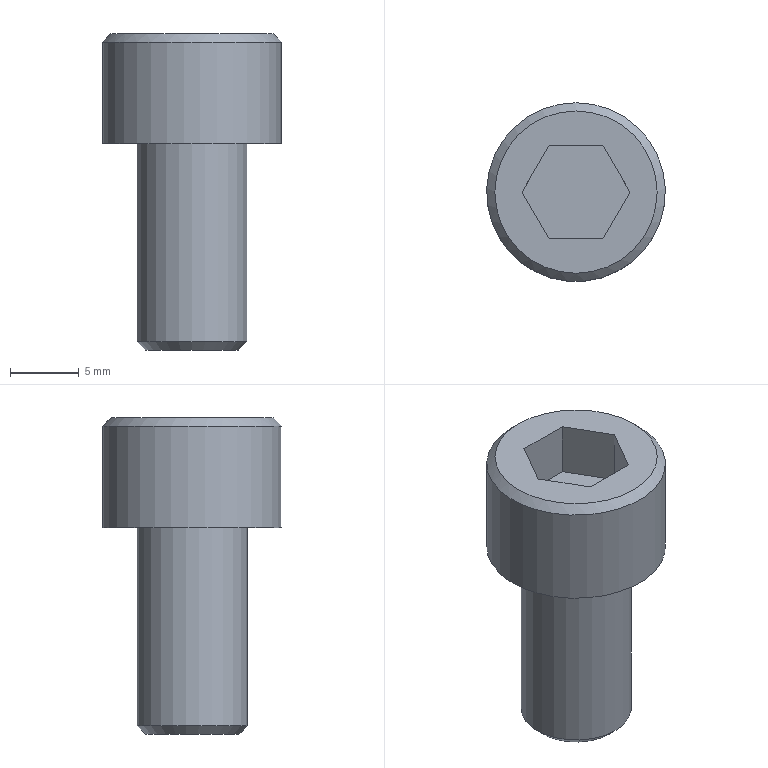Part | STEP file | M8.00-15.00 | 1 solid | 14 faces | box 13 x 13 x 23 mm | volume 1644 mm3 | plane 10 | cylinder 2 | cone 2 | commonest cylinder face diameters 8 x1 13 x1